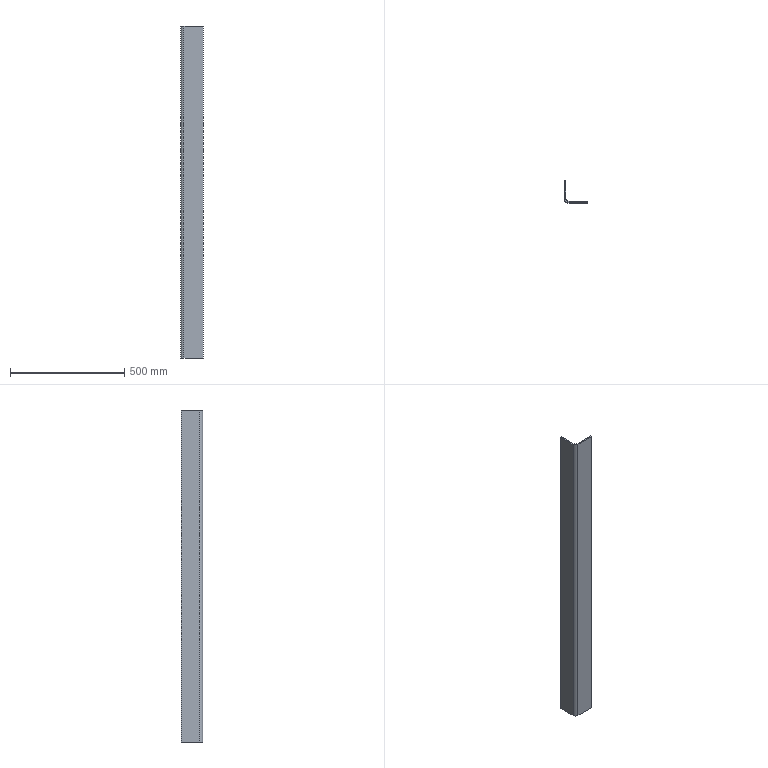Part | STEP file | _20002 | 1 solid | 10 faces | box 100 x 94 x 1450 mm | volume 1590791 mm3 | plane 8 | cylinder 2 | commonest cylinder face diameters 18 x1 30 x1
STEP:
#1=CARTESIAN_POINT('',(50.,-100.,-725.));
#2=VERTEX_POINT('',#1);
#3=CARTESIAN_POINT('',(50.,-100.,725.));
#4=VERTEX_POINT('',#3);
#5=CARTESIAN_POINT('',(50.,-100.,-725.));
#6=DIRECTION('',(0.,0.,1.));
#7=VECTOR('',#6,1000.);
#8=LINE('',#5,#7);
#9=EDGE_CURVE('',#2,#4,#8,.T.);
#10=ORIENTED_EDGE('',*,*,#9,.T.);
#11=CARTESIAN_POINT('',(-35.,-100.,725.));
#12=VERTEX_POINT('',#11);
#13=CARTESIAN_POINT('',(50.,-100.,725.));
#14=DIRECTION('',(-1.,0.,0.));
#15=VECTOR('',#14,1000.);
#16=LINE('',#13,#15);
#17=EDGE_CURVE('',#4,#12,#16,.T.);
#18=ORIENTED_EDGE('',*,*,#17,.T.);
#19=CARTESIAN_POINT('',(-35.,-100.,-725.));
#20=VERTEX_POINT('',#19);
#21=CARTESIAN_POINT('',(-35.,-100.,-725.));
#22=DIRECTION('',(0.,0.,1.));
#23=VECTOR('',#22,1000.);
#24=LINE('',#21,#23);
#25=EDGE_CURVE('',#20,#12,#24,.T.);
#26=ORIENTED_EDGE('',*,*,#25,.F.);
#27=CARTESIAN_POINT('',(50.,-100.,-725.));
#28=DIRECTION('',(-1.,0.,0.));
#29=VECTOR('',#28,1000.);
#30=LINE('',#27,#29);
#31=EDGE_CURVE('',#2,#20,#30,.T.);
#32=ORIENTED_EDGE('',*,*,#31,.F.);
#33=EDGE_LOOP('',(#10,#18,#26,#32));
#34=FACE_OUTER_BOUND('',#33,.T.);
#35=CARTESIAN_POINT('',(-50.,-100.,725.));
#36=DIRECTION('',(0.,1.,0.));
#37=DIRECTION('',(1.,0.,0.));
#38=AXIS2_PLACEMENT_3D('',#35,#36,#37);
#39=PLANE('',#38);
#40=ADVANCED_FACE('',(#34),#39,.F.);
#41=CARTESIAN_POINT('',(50.,-94.,-725.));
#42=VERTEX_POINT('',#41);
#43=CARTESIAN_POINT('',(50.,-94.,725.));
#44=VERTEX_POINT('',#43);
#45=CARTESIAN_POINT('',(50.,-94.,-725.));
#46=DIRECTION('',(0.,0.,1.));
#47=VECTOR('',#46,1000.);
#48=LINE('',#45,#47);
#49=EDGE_CURVE('',#42,#44,#48,.T.);
#50=ORIENTED_EDGE('',*,*,#49,.T.);
#51=CARTESIAN_POINT('',(50.,-100.,725.));
#52=DIRECTION('',(0.,1.,0.));
#53=VECTOR('',#52,1000.);
#54=LINE('',#51,#53);
#55=EDGE_CURVE('',#4,#44,#54,.T.);
#56=ORIENTED_EDGE('',*,*,#55,.F.);
#57=ORIENTED_EDGE('',*,*,#9,.F.);
#58=CARTESIAN_POINT('',(50.,-100.,-725.));
#59=DIRECTION('',(0.,1.,0.));
#60=VECTOR('',#59,1000.);
#61=LINE('',#58,#60);
#62=EDGE_CURVE('',#2,#42,#61,.T.);
#63=ORIENTED_EDGE('',*,*,#62,.T.);
#64=EDGE_LOOP('',(#50,#56,#57,#63));
#65=FACE_OUTER_BOUND('',#64,.T.);
#66=CARTESIAN_POINT('',(50.,-94.,725.));
#67=DIRECTION('',(1.,0.,0.));
#68=DIRECTION('',(0.,1.,0.));
#69=AXIS2_PLACEMENT_3D('',#66,#67,#68);
#70=PLANE('',#69);
#71=ADVANCED_FACE('',(#65),#70,.T.);
#72=CARTESIAN_POINT('',(-35.,-94.,725.));
#73=VERTEX_POINT('',#72);
#74=CARTESIAN_POINT('',(-35.,-94.,-725.));
#75=VERTEX_POINT('',#74);
#76=CARTESIAN_POINT('',(-35.,-94.,725.));
#77=DIRECTION('',(0.,0.,-1.));
#78=VECTOR('',#77,1000.);
#79=LINE('',#76,#78);
#80=EDGE_CURVE('',#73,#75,#79,.T.);
#81=ORIENTED_EDGE('',*,*,#80,.F.);
#82=CARTESIAN_POINT('',(50.,-94.,725.));
#83=DIRECTION('',(-1.,0.,0.));
#84=VECTOR('',#83,1000.);
#85=LINE('',#82,#84);
#86=EDGE_CURVE('',#44,#73,#85,.T.);
#87=ORIENTED_EDGE('',*,*,#86,.F.);
#88=ORIENTED_EDGE('',*,*,#49,.F.);
#89=CARTESIAN_POINT('',(50.,-94.,-725.));
#90=DIRECTION('',(-1.,0.,0.));
#91=VECTOR('',#90,1000.);
#92=LINE('',#89,#91);
#93=EDGE_CURVE('',#42,#75,#92,.T.);
#94=ORIENTED_EDGE('',*,*,#93,.T.);
#95=EDGE_LOOP('',(#81,#87,#88,#94));
#96=FACE_OUTER_BOUND('',#95,.T.);
#97=CARTESIAN_POINT('',(-50.,-94.,725.));
#98=DIRECTION('',(0.,1.,0.));
#99=DIRECTION('',(1.,0.,0.));
#100=AXIS2_PLACEMENT_3D('',#97,#98,#99);
#101=PLANE('',#100);
#102=ADVANCED_FACE('',(#96),#101,.T.);
#103=CARTESIAN_POINT('',(-44.,-6.,725.));
#104=VERTEX_POINT('',#103);
#105=CARTESIAN_POINT('',(-50.,-6.,725.));
#106=VERTEX_POINT('',#105);
#107=CARTESIAN_POINT('',(-44.,-6.,725.));
#108=DIRECTION('',(-1.,0.,0.));
#109=VECTOR('',#108,1000.);
#110=LINE('',#107,#109);
#111=EDGE_CURVE('',#104,#106,#110,.T.);
#112=ORIENTED_EDGE('',*,*,#111,.T.);
#113=CARTESIAN_POINT('',(-50.,-85.,725.));
#114=VERTEX_POINT('',#113);
#115=CARTESIAN_POINT('',(-50.,-85.,725.));
#116=DIRECTION('',(0.,1.,0.));
#117=VECTOR('',#116,1000.);
#118=LINE('',#115,#117);
#119=EDGE_CURVE('',#114,#106,#118,.T.);
#120=ORIENTED_EDGE('',*,*,#119,.F.);
#121=CARTESIAN_POINT('',(-35.,-85.,725.));
#122=DIRECTION('',(0.,0.,1.));
#123=DIRECTION('',(-1.,0.,0.));
#124=AXIS2_PLACEMENT_3D('',#121,#122,#123);
#125=CIRCLE('',#124,15.);
#126=EDGE_CURVE('',#114,#12,#125,.T.);
#127=ORIENTED_EDGE('',*,*,#126,.T.);
#128=ORIENTED_EDGE('',*,*,#17,.F.);
#129=ORIENTED_EDGE('',*,*,#55,.T.);
#130=ORIENTED_EDGE('',*,*,#86,.T.);
#131=CARTESIAN_POINT('',(-44.,-85.,725.));
#132=VERTEX_POINT('',#131);
#133=CARTESIAN_POINT('',(-35.,-85.,725.));
#134=DIRECTION('',(0.,0.,-1.));
#135=DIRECTION('',(0.,-1.,0.));
#136=AXIS2_PLACEMENT_3D('',#133,#134,#135);
#137=CIRCLE('',#136,9.);
#138=EDGE_CURVE('',#73,#132,#137,.T.);
#139=ORIENTED_EDGE('',*,*,#138,.T.);
#140=CARTESIAN_POINT('',(-44.,-85.,725.));
#141=DIRECTION('',(0.,1.,0.));
#142=VECTOR('',#141,1000.);
#143=LINE('',#140,#142);
#144=EDGE_CURVE('',#132,#104,#143,.T.);
#145=ORIENTED_EDGE('',*,*,#144,.T.);
#146=EDGE_LOOP('',(#112,#120,#127,#128,#129,#130,#139,#145));
#147=FACE_OUTER_BOUND('',#146,.T.);
#148=CARTESIAN_POINT('',(-35.,-85.,725.));
#149=DIRECTION('',(0.,0.,1.));
#150=DIRECTION('',(1.,0.,0.));
#151=AXIS2_PLACEMENT_3D('',#148,#149,#150);
#152=PLANE('',#151);
#153=ADVANCED_FACE('',(#147),#152,.T.);
#154=CARTESIAN_POINT('',(-44.,-6.,-725.));
#155=VERTEX_POINT('',#154);
#156=CARTESIAN_POINT('',(-44.,-6.,-725.));
#157=DIRECTION('',(0.,0.,1.));
#158=VECTOR('',#157,1000.);
#159=LINE('',#156,#158);
#160=EDGE_CURVE('',#155,#104,#159,.T.);
#161=ORIENTED_EDGE('',*,*,#160,.T.);
#162=ORIENTED_EDGE('',*,*,#144,.F.);
#163=CARTESIAN_POINT('',(-44.,-85.,-725.));
#164=VERTEX_POINT('',#163);
#165=CARTESIAN_POINT('',(-44.,-85.,-725.));
#166=DIRECTION('',(0.,0.,1.));
#167=VECTOR('',#166,1000.);
#168=LINE('',#165,#167);
#169=EDGE_CURVE('',#164,#132,#168,.T.);
#170=ORIENTED_EDGE('',*,*,#169,.F.);
#171=CARTESIAN_POINT('',(-44.,-85.,-725.));
#172=DIRECTION('',(0.,1.,0.));
#173=VECTOR('',#172,1000.);
#174=LINE('',#171,#173);
#175=EDGE_CURVE('',#164,#155,#174,.T.);
#176=ORIENTED_EDGE('',*,*,#175,.T.);
#177=EDGE_LOOP('',(#161,#162,#170,#176));
#178=FACE_OUTER_BOUND('',#177,.T.);
#179=CARTESIAN_POINT('',(-44.,-8.,725.));
#180=DIRECTION('',(1.,0.,0.));
#181=DIRECTION('',(0.,1.,0.));
#182=AXIS2_PLACEMENT_3D('',#179,#180,#181);
#183=PLANE('',#182);
#184=ADVANCED_FACE('',(#178),#183,.T.);
#185=CARTESIAN_POINT('',(-50.,-6.,-725.));
#186=VERTEX_POINT('',#185);
#187=CARTESIAN_POINT('',(-50.,-6.,-725.));
#188=DIRECTION('',(0.,0.,1.));
#189=VECTOR('',#188,1000.);
#190=LINE('',#187,#189);
#191=EDGE_CURVE('',#186,#106,#190,.T.);
#192=ORIENTED_EDGE('',*,*,#191,.T.);
#193=ORIENTED_EDGE('',*,*,#111,.F.);
#194=ORIENTED_EDGE('',*,*,#160,.F.);
#195=CARTESIAN_POINT('',(-44.,-6.,-725.));
#196=DIRECTION('',(-1.,0.,0.));
#197=VECTOR('',#196,1000.);
#198=LINE('',#195,#197);
#199=EDGE_CURVE('',#155,#186,#198,.T.);
#200=ORIENTED_EDGE('',*,*,#199,.T.);
#201=EDGE_LOOP('',(#192,#193,#194,#200));
#202=FACE_OUTER_BOUND('',#201,.T.);
#203=CARTESIAN_POINT('',(-50.,-6.,725.));
#204=DIRECTION('',(0.,1.,0.));
#205=DIRECTION('',(1.,0.,0.));
#206=AXIS2_PLACEMENT_3D('',#203,#204,#205);
#207=PLANE('',#206);
#208=ADVANCED_FACE('',(#202),#207,.T.);
#209=CARTESIAN_POINT('',(-50.,-85.,-725.));
#210=VERTEX_POINT('',#209);
#211=CARTESIAN_POINT('',(-50.,-85.,725.));
#212=DIRECTION('',(0.,0.,-1.));
#213=VECTOR('',#212,1000.);
#214=LINE('',#211,#213);
#215=EDGE_CURVE('',#114,#210,#214,.T.);
#216=ORIENTED_EDGE('',*,*,#215,.F.);
#217=ORIENTED_EDGE('',*,*,#119,.T.);
#218=ORIENTED_EDGE('',*,*,#191,.F.);
#219=CARTESIAN_POINT('',(-50.,-85.,-725.));
#220=DIRECTION('',(0.,1.,0.));
#221=VECTOR('',#220,1000.);
#222=LINE('',#219,#221);
#223=EDGE_CURVE('',#210,#186,#222,.T.);
#224=ORIENTED_EDGE('',*,*,#223,.F.);
#225=EDGE_LOOP('',(#216,#217,#218,#224));
#226=FACE_OUTER_BOUND('',#225,.T.);
#227=CARTESIAN_POINT('',(-50.,-8.,725.));
#228=DIRECTION('',(1.,0.,0.));
#229=DIRECTION('',(0.,1.,0.));
#230=AXIS2_PLACEMENT_3D('',#227,#228,#229);
#231=PLANE('',#230);
#232=ADVANCED_FACE('',(#226),#231,.F.);
#233=ORIENTED_EDGE('',*,*,#25,.T.);
#234=ORIENTED_EDGE('',*,*,#126,.F.);
#235=ORIENTED_EDGE('',*,*,#215,.T.);
#236=CARTESIAN_POINT('',(-35.,-85.,-725.));
#237=DIRECTION('',(0.,0.,-1.));
#238=DIRECTION('',(0.,-1.,0.));
#239=AXIS2_PLACEMENT_3D('',#236,#237,#238);
#240=CIRCLE('',#239,15.);
#241=EDGE_CURVE('',#20,#210,#240,.T.);
#242=ORIENTED_EDGE('',*,*,#241,.F.);
#243=EDGE_LOOP('',(#233,#234,#235,#242));
#244=FACE_OUTER_BOUND('',#243,.T.);
#245=CARTESIAN_POINT('',(-35.,-85.,725.));
#246=DIRECTION('',(0.,0.,-1.));
#247=DIRECTION('',(-1.,0.,0.));
#248=AXIS2_PLACEMENT_3D('',#245,#246,#247);
#249=CYLINDRICAL_SURFACE('',#248,15.);
#250=ADVANCED_FACE('',(#244),#249,.T.);
#251=ORIENTED_EDGE('',*,*,#223,.T.);
#252=ORIENTED_EDGE('',*,*,#199,.F.);
#253=ORIENTED_EDGE('',*,*,#175,.F.);
#254=CARTESIAN_POINT('',(-35.,-85.,-725.));
#255=DIRECTION('',(0.,0.,1.));
#256=DIRECTION('',(-1.,0.,0.));
#257=AXIS2_PLACEMENT_3D('',#254,#255,#256);
#258=CIRCLE('',#257,9.);
#259=EDGE_CURVE('',#164,#75,#258,.T.);
#260=ORIENTED_EDGE('',*,*,#259,.T.);
#261=ORIENTED_EDGE('',*,*,#93,.F.);
#262=ORIENTED_EDGE('',*,*,#62,.F.);
#263=ORIENTED_EDGE('',*,*,#31,.T.);
#264=ORIENTED_EDGE('',*,*,#241,.T.);
#265=EDGE_LOOP('',(#251,#252,#253,#260,#261,#262,#263,#264));
#266=FACE_OUTER_BOUND('',#265,.T.);
#267=CARTESIAN_POINT('',(-35.,-100.,-725.));
#268=DIRECTION('',(0.,0.,-1.));
#269=DIRECTION('',(0.,-1.,0.));
#270=AXIS2_PLACEMENT_3D('',#267,#268,#269);
#271=PLANE('',#270);
#272=ADVANCED_FACE('',(#266),#271,.T.);
#273=ORIENTED_EDGE('',*,*,#169,.T.);
#274=ORIENTED_EDGE('',*,*,#138,.F.);
#275=ORIENTED_EDGE('',*,*,#80,.T.);
#276=ORIENTED_EDGE('',*,*,#259,.F.);
#277=EDGE_LOOP('',(#273,#274,#275,#276));
#278=FACE_OUTER_BOUND('',#277,.T.);
#279=CARTESIAN_POINT('',(-35.,-85.,725.));
#280=DIRECTION('',(0.,0.,-1.));
#281=DIRECTION('',(-1.,0.,0.));
#282=AXIS2_PLACEMENT_3D('',#279,#280,#281);
#283=CYLINDRICAL_SURFACE('',#282,9.);
#284=ADVANCED_FACE('',(#278),#283,.F.);
#285=CLOSED_SHELL('',(#40,#71,#102,#153,#184,#208,#232,#250,#272,#284));
#286=MANIFOLD_SOLID_BREP('',#285);
#287=CARTESIAN_POINT('',(0.,0.,0.));
#288=DIRECTION('',(0.,0.,1.));
#289=DIRECTION('',(1.,0.,0.));
#290=AXIS2_PLACEMENT_3D('',#287,#288,#289);
#291=(LENGTH_UNIT()NAMED_UNIT(*)SI_UNIT(.MILLI.,.METRE.));
#292=UNCERTAINTY_MEASURE_WITH_UNIT(LENGTH_MEASURE(0.00001),#291,'','');
#293=(NAMED_UNIT(*)PLANE_ANGLE_UNIT()SI_UNIT($,.RADIAN.));
#294=(NAMED_UNIT(*)SI_UNIT($,.STERADIAN.)SOLID_ANGLE_UNIT());
#295=(GEOMETRIC_REPRESENTATION_CONTEXT(3)GLOBAL_UNCERTAINTY_ASSIGNED_CONTEXT((#292))GLOBAL_UNIT_ASSIGNED_CONTEXT((#291,#293,#294))REPRESENTATION_CONTEXT('',''));
#296=ADVANCED_BREP_SHAPE_REPRESENTATION('',(#286,#290),#295);